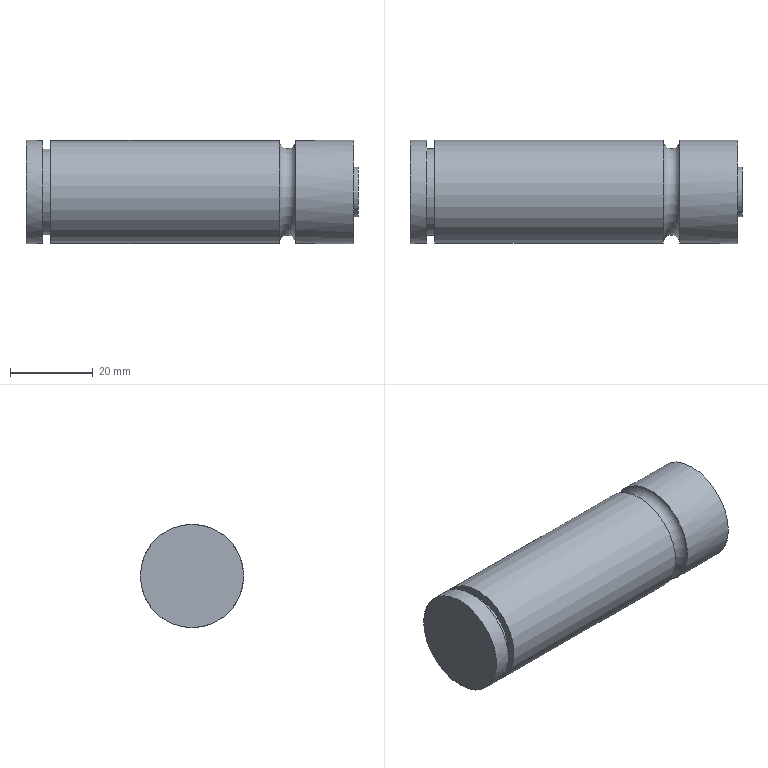Part | NX | features MAIN_BODY 2 | 1 solid | 11 faces | box 80.1 x 24.9 x 24.9 mm | volume 37885 mm3 | cylinder 5 | plane 5 | torus 1 | commonest cylinder face diameters 24.9 x3 12 x1 20.9 x1
STEP:
#1=CARTESIAN_POINT('',(-227.6,-81.05,-140.));
#2=VERTEX_POINT('',#1);
#3=CARTESIAN_POINT('',(-227.6,-93.5,-140.));
#4=DIRECTION('',(1.,0.,0.));
#5=DIRECTION('',(0.,1.,0.));
#6=AXIS2_PLACEMENT_3D('',#3,#4,#5);
#7=CIRCLE('',#6,12.45);
#8=EDGE_CURVE('',#2,#2,#7,.F.);
#9=ORIENTED_EDGE('',*,*,#8,.F.);
#10=EDGE_LOOP('',(#9));
#11=FACE_BOUND('',#10,.T.);
#12=CARTESIAN_POINT('',(-172.5,-81.05,-140.));
#13=VERTEX_POINT('',#12);
#14=CARTESIAN_POINT('',(-172.5,-93.5,-140.));
#15=DIRECTION('',(1.,0.,0.));
#16=DIRECTION('',(0.,1.,0.));
#17=AXIS2_PLACEMENT_3D('',#14,#15,#16);
#18=CIRCLE('',#17,12.45);
#19=EDGE_CURVE('',#13,#13,#18,.T.);
#20=ORIENTED_EDGE('',*,*,#19,.F.);
#21=EDGE_LOOP('',(#20));
#22=FACE_BOUND('',#21,.T.);
#23=CARTESIAN_POINT('',(-154.5,-93.5,-140.));
#24=DIRECTION('',(-1.,0.,0.));
#25=DIRECTION('',(0.,1.,0.));
#26=AXIS2_PLACEMENT_3D('',#23,#24,#25);
#27=CYLINDRICAL_SURFACE('',#26,12.45);
#28=ADVANCED_FACE('',(#11,#22),#27,.T.);
#29=CARTESIAN_POINT('',(-154.5,-105.95,-140.));
#30=VERTEX_POINT('',#29);
#31=CARTESIAN_POINT('',(-154.5,-93.5,-140.));
#32=DIRECTION('',(-1.,0.,0.));
#33=DIRECTION('',(0.,-1.,0.));
#34=AXIS2_PLACEMENT_3D('',#31,#32,#33);
#35=CIRCLE('',#34,12.45);
#36=EDGE_CURVE('',#30,#30,#35,.T.);
#37=ORIENTED_EDGE('',*,*,#36,.F.);
#38=EDGE_LOOP('',(#37));
#39=FACE_BOUND('',#38,.T.);
#40=CARTESIAN_POINT('',(-154.5,-99.5,-140.));
#41=VERTEX_POINT('',#40);
#42=CARTESIAN_POINT('',(-154.5,-93.5,-140.));
#43=DIRECTION('',(-1.,0.,0.));
#44=DIRECTION('',(0.,-1.,0.));
#45=AXIS2_PLACEMENT_3D('',#42,#43,#44);
#46=CIRCLE('',#45,6.);
#47=EDGE_CURVE('',#41,#41,#46,.T.);
#48=ORIENTED_EDGE('',*,*,#47,.T.);
#49=EDGE_LOOP('',(#48));
#50=FACE_BOUND('',#49,.T.);
#51=CARTESIAN_POINT('',(-154.5,-93.5,-140.));
#52=DIRECTION('',(1.,0.,0.));
#53=DIRECTION('',(0.,-1.,0.));
#54=AXIS2_PLACEMENT_3D('',#51,#52,#53);
#55=PLANE('',#54);
#56=ADVANCED_FACE('',(#39,#50),#55,.T.);
#57=CARTESIAN_POINT('',(-168.5,-81.05,-140.));
#58=VERTEX_POINT('',#57);
#59=CARTESIAN_POINT('',(-168.5,-93.5,-140.));
#60=DIRECTION('',(1.,0.,0.));
#61=DIRECTION('',(0.,1.,0.));
#62=AXIS2_PLACEMENT_3D('',#59,#60,#61);
#63=CIRCLE('',#62,12.45);
#64=EDGE_CURVE('',#58,#58,#63,.F.);
#65=ORIENTED_EDGE('',*,*,#64,.F.);
#66=EDGE_LOOP('',(#65));
#67=FACE_BOUND('',#66,.T.);
#68=ORIENTED_EDGE('',*,*,#36,.T.);
#69=EDGE_LOOP('',(#68));
#70=FACE_BOUND('',#69,.T.);
#71=CARTESIAN_POINT('',(-154.5,-93.5,-140.));
#72=DIRECTION('',(-1.,0.,0.));
#73=DIRECTION('',(0.,1.,0.));
#74=AXIS2_PLACEMENT_3D('',#71,#72,#73);
#75=CYLINDRICAL_SURFACE('',#74,12.45);
#76=ADVANCED_FACE('',(#67,#70),#75,.T.);
#77=CARTESIAN_POINT('',(-153.5,-99.5,-140.));
#78=VERTEX_POINT('',#77);
#79=CARTESIAN_POINT('',(-153.5,-93.5,-140.));
#80=DIRECTION('',(-1.,0.,0.));
#81=DIRECTION('',(0.,-1.,0.));
#82=AXIS2_PLACEMENT_3D('',#79,#80,#81);
#83=CIRCLE('',#82,6.);
#84=EDGE_CURVE('',#78,#78,#83,.T.);
#85=ORIENTED_EDGE('',*,*,#84,.T.);
#86=EDGE_LOOP('',(#85));
#87=FACE_BOUND('',#86,.T.);
#88=ORIENTED_EDGE('',*,*,#47,.F.);
#89=EDGE_LOOP('',(#88));
#90=FACE_BOUND('',#89,.T.);
#91=CARTESIAN_POINT('',(-153.5,-93.5,-140.));
#92=DIRECTION('',(-1.,0.,0.));
#93=DIRECTION('',(0.,1.,0.));
#94=AXIS2_PLACEMENT_3D('',#91,#92,#93);
#95=CYLINDRICAL_SURFACE('',#94,6.);
#96=ADVANCED_FACE('',(#87,#90),#95,.T.);
#97=ORIENTED_EDGE('',*,*,#84,.F.);
#98=EDGE_LOOP('',(#97));
#99=FACE_BOUND('',#98,.T.);
#100=CARTESIAN_POINT('',(-153.5,-93.5,-140.));
#101=DIRECTION('',(1.,0.,0.));
#102=DIRECTION('',(0.,-1.,0.));
#103=AXIS2_PLACEMENT_3D('',#100,#101,#102);
#104=PLANE('',#103);
#105=ADVANCED_FACE('',(#99),#104,.T.);
#106=ORIENTED_EDGE('',*,*,#64,.T.);
#107=EDGE_LOOP('',(#106));
#108=FACE_BOUND('',#107,.T.);
#109=ORIENTED_EDGE('',*,*,#19,.T.);
#110=EDGE_LOOP('',(#109));
#111=FACE_BOUND('',#110,.T.);
#112=CARTESIAN_POINT('',(-170.5,-93.5,-140.));
#113=DIRECTION('',(-1.,0.,0.));
#114=DIRECTION('',(0.,1.,0.));
#115=AXIS2_PLACEMENT_3D('',#112,#113,#114);
#116=TOROIDAL_SURFACE('',#115,12.45,2.);
#117=ADVANCED_FACE('',(#108,#111),#116,.F.);
#118=CARTESIAN_POINT('',(-227.6,-103.95,-140.));
#119=VERTEX_POINT('',#118);
#120=CARTESIAN_POINT('',(-227.6,-93.5,-140.));
#121=DIRECTION('',(-1.,0.,0.));
#122=DIRECTION('',(0.,-1.,0.));
#123=AXIS2_PLACEMENT_3D('',#120,#121,#122);
#124=CIRCLE('',#123,10.45);
#125=EDGE_CURVE('',#119,#119,#124,.T.);
#126=ORIENTED_EDGE('',*,*,#125,.F.);
#127=EDGE_LOOP('',(#126));
#128=FACE_BOUND('',#127,.T.);
#129=ORIENTED_EDGE('',*,*,#8,.T.);
#130=EDGE_LOOP('',(#129));
#131=FACE_BOUND('',#130,.T.);
#132=CARTESIAN_POINT('',(-227.6,-93.5,-140.));
#133=DIRECTION('',(-1.,0.,0.));
#134=DIRECTION('',(0.,1.,0.));
#135=AXIS2_PLACEMENT_3D('',#132,#133,#134);
#136=PLANE('',#135);
#137=ADVANCED_FACE('',(#128,#131),#136,.T.);
#138=CARTESIAN_POINT('',(-229.6,-103.95,-140.));
#139=VERTEX_POINT('',#138);
#140=CARTESIAN_POINT('',(-229.6,-93.5,-140.));
#141=DIRECTION('',(-1.,0.,0.));
#142=DIRECTION('',(0.,-1.,0.));
#143=AXIS2_PLACEMENT_3D('',#140,#141,#142);
#144=CIRCLE('',#143,10.45);
#145=EDGE_CURVE('',#139,#139,#144,.T.);
#146=ORIENTED_EDGE('',*,*,#145,.T.);
#147=EDGE_LOOP('',(#146));
#148=FACE_BOUND('',#147,.T.);
#149=CARTESIAN_POINT('',(-229.6,-81.05,-140.));
#150=VERTEX_POINT('',#149);
#151=CARTESIAN_POINT('',(-229.6,-93.5,-140.));
#152=DIRECTION('',(1.,0.,0.));
#153=DIRECTION('',(0.,1.,0.));
#154=AXIS2_PLACEMENT_3D('',#151,#152,#153);
#155=CIRCLE('',#154,12.45);
#156=EDGE_CURVE('',#150,#150,#155,.T.);
#157=ORIENTED_EDGE('',*,*,#156,.T.);
#158=EDGE_LOOP('',(#157));
#159=FACE_BOUND('',#158,.T.);
#160=CARTESIAN_POINT('',(-229.6,-93.5,-140.));
#161=DIRECTION('',(-1.,0.,0.));
#162=DIRECTION('',(0.,1.,0.));
#163=AXIS2_PLACEMENT_3D('',#160,#161,#162);
#164=PLANE('',#163);
#165=ADVANCED_FACE('',(#148,#159),#164,.F.);
#166=ORIENTED_EDGE('',*,*,#125,.T.);
#167=EDGE_LOOP('',(#166));
#168=FACE_BOUND('',#167,.T.);
#169=ORIENTED_EDGE('',*,*,#145,.F.);
#170=EDGE_LOOP('',(#169));
#171=FACE_BOUND('',#170,.T.);
#172=CARTESIAN_POINT('',(-229.6,-93.5,-140.));
#173=DIRECTION('',(1.,0.,0.));
#174=DIRECTION('',(0.,-1.,0.));
#175=AXIS2_PLACEMENT_3D('',#172,#173,#174);
#176=CYLINDRICAL_SURFACE('',#175,10.45);
#177=ADVANCED_FACE('',(#168,#171),#176,.T.);
#178=CARTESIAN_POINT('',(-233.6,-105.95,-140.));
#179=VERTEX_POINT('',#178);
#180=CARTESIAN_POINT('',(-233.6,-93.5,-140.));
#181=DIRECTION('',(-1.,0.,0.));
#182=DIRECTION('',(0.,-1.,0.));
#183=AXIS2_PLACEMENT_3D('',#180,#181,#182);
#184=CIRCLE('',#183,12.45);
#185=EDGE_CURVE('',#179,#179,#184,.T.);
#186=ORIENTED_EDGE('',*,*,#185,.T.);
#187=EDGE_LOOP('',(#186));
#188=FACE_BOUND('',#187,.T.);
#189=CARTESIAN_POINT('',(-233.6,-93.5,-140.));
#190=DIRECTION('',(1.,0.,0.));
#191=DIRECTION('',(0.,-1.,0.));
#192=AXIS2_PLACEMENT_3D('',#189,#190,#191);
#193=PLANE('',#192);
#194=ADVANCED_FACE('',(#188),#193,.F.);
#195=ORIENTED_EDGE('',*,*,#156,.F.);
#196=EDGE_LOOP('',(#195));
#197=FACE_BOUND('',#196,.T.);
#198=ORIENTED_EDGE('',*,*,#185,.F.);
#199=EDGE_LOOP('',(#198));
#200=FACE_BOUND('',#199,.T.);
#201=CARTESIAN_POINT('',(-154.5,-93.5,-140.));
#202=DIRECTION('',(-1.,0.,0.));
#203=DIRECTION('',(0.,1.,0.));
#204=AXIS2_PLACEMENT_3D('',#201,#202,#203);
#205=CYLINDRICAL_SURFACE('',#204,12.45);
#206=ADVANCED_FACE('',(#197,#200),#205,.T.);
#207=CLOSED_SHELL('',(#28,#56,#76,#96,#105,#117,#137,#165,#177,#194,#206));
#208=MANIFOLD_SOLID_BREP('',#207);
#209=(LENGTH_UNIT()NAMED_UNIT(*)SI_UNIT(.MILLI.,.METRE.));
#210=UNCERTAINTY_MEASURE_WITH_UNIT(LENGTH_MEASURE(0.00001),#209,'','');
#211=(NAMED_UNIT(*)PLANE_ANGLE_UNIT()SI_UNIT($,.RADIAN.));
#212=(NAMED_UNIT(*)SI_UNIT($,.STERADIAN.)SOLID_ANGLE_UNIT());
#213=(GEOMETRIC_REPRESENTATION_CONTEXT(3)GLOBAL_UNCERTAINTY_ASSIGNED_CONTEXT((#210))GLOBAL_UNIT_ASSIGNED_CONTEXT((#209,#211,#212))REPRESENTATION_CONTEXT('',''));
#214=ADVANCED_BREP_SHAPE_REPRESENTATION('',(#208),#213);